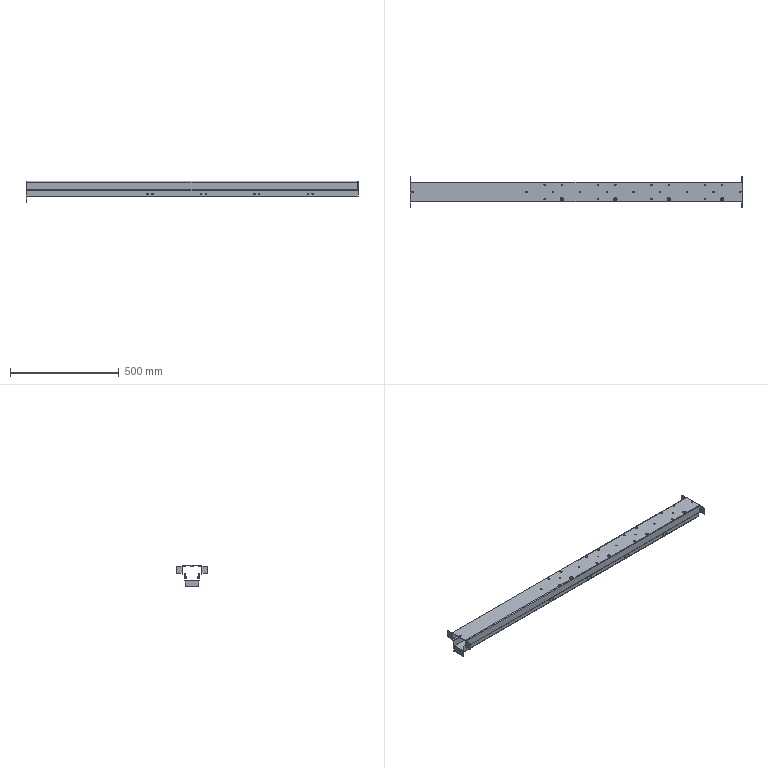Part | SolidWorks | features BaseBody 1 | 1 solid | 552 faces | box 1528 x 146 x 98 mm | volume 1194615 mm3 | plane 364 | cylinder 188 | commonest cylinder face diameters 6 x96 6.5 x68 1 x12 16 x8 4 x4